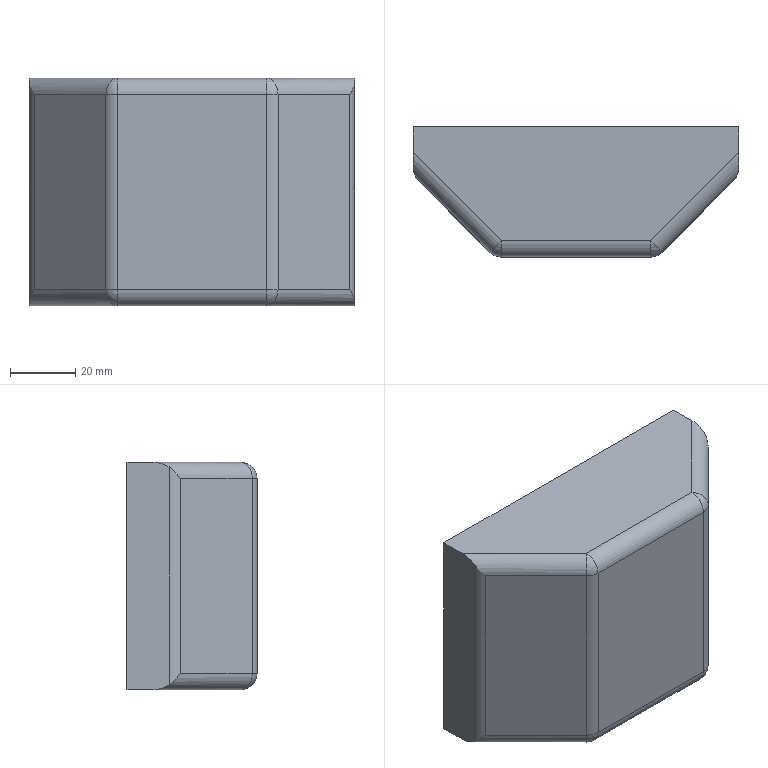Part | SolidWorks | features Extrusion 1, Fillet 1 | 1 solid | 22 faces | box 100 x 40 x 70 mm | volume 234811 mm3 | cylinder 10 | plane 8 | sphere 4 | commonest cylinder face diameters 10 x10
STEP:
#1=CARTESIAN_POINT('',(0.,-12.929,1.464));
#2=VERTEX_POINT('',#1);
#3=CARTESIAN_POINT('',(0.,-12.929,68.536));
#4=VERTEX_POINT('',#3);
#5=CARTESIAN_POINT('',(0.,-12.929,70.));
#6=DIRECTION('',(0.,0.,1.));
#7=VECTOR('',#6,1000.);
#8=LINE('',#5,#7);
#9=EDGE_CURVE('',#2,#4,#8,.T.);
#10=ORIENTED_EDGE('',*,*,#9,.T.);
#11=CARTESIAN_POINT('',(0.,-7.929,70.));
#12=VERTEX_POINT('',#11);
#13=CARTESIAN_POINT('',(0.,-12.929,68.536));
#14=CARTESIAN_POINT('',(0.,-11.585,69.486));
#15=CARTESIAN_POINT('',(0.,-9.829,70.));
#16=CARTESIAN_POINT('',(0.,-7.929,70.));
#17=(BOUNDED_CURVE()B_SPLINE_CURVE(3,(#13,#14,#15,#16),.UNSPECIFIED.,.F.,.F.)B_SPLINE_CURVE_WITH_KNOTS((4,4),(0.7854,1.571),.UNSPECIFIED.)CURVE()GEOMETRIC_REPRESENTATION_ITEM()RATIONAL_B_SPLINE_CURVE((1.,0.9493,0.9493,1.))REPRESENTATION_ITEM(''));
#18=EDGE_CURVE('',#4,#12,#17,.T.);
#19=ORIENTED_EDGE('',*,*,#18,.T.);
#20=CARTESIAN_POINT('',(0.,0.,70.));
#21=VERTEX_POINT('',#20);
#22=CARTESIAN_POINT('',(0.,0.,70.));
#23=DIRECTION('',(0.,-1.,0.));
#24=VECTOR('',#23,1000.);
#25=LINE('',#22,#24);
#26=EDGE_CURVE('',#21,#12,#25,.T.);
#27=ORIENTED_EDGE('',*,*,#26,.F.);
#28=CARTESIAN_POINT('',(0.,0.,0.));
#29=VERTEX_POINT('',#28);
#30=CARTESIAN_POINT('',(0.,0.,70.));
#31=DIRECTION('',(0.,0.,-1.));
#32=VECTOR('',#31,1000.);
#33=LINE('',#30,#32);
#34=EDGE_CURVE('',#21,#29,#33,.T.);
#35=ORIENTED_EDGE('',*,*,#34,.T.);
#36=CARTESIAN_POINT('',(0.,-7.929,0.));
#37=VERTEX_POINT('',#36);
#38=CARTESIAN_POINT('',(0.,0.,0.));
#39=DIRECTION('',(0.,-1.,0.));
#40=VECTOR('',#39,1000.);
#41=LINE('',#38,#40);
#42=EDGE_CURVE('',#29,#37,#41,.T.);
#43=ORIENTED_EDGE('',*,*,#42,.T.);
#44=CARTESIAN_POINT('',(0.,-7.929,0.));
#45=CARTESIAN_POINT('',(0.,-9.829,0.));
#46=CARTESIAN_POINT('',(0.,-11.585,0.5143));
#47=CARTESIAN_POINT('',(0.,-12.929,1.464));
#48=(BOUNDED_CURVE()B_SPLINE_CURVE(3,(#44,#45,#46,#47),.UNSPECIFIED.,.F.,.F.)B_SPLINE_CURVE_WITH_KNOTS((4,4),(1.571,2.356),.UNSPECIFIED.)CURVE()GEOMETRIC_REPRESENTATION_ITEM()RATIONAL_B_SPLINE_CURVE((1.,0.9493,0.9493,1.))REPRESENTATION_ITEM(''));
#49=EDGE_CURVE('',#37,#2,#48,.T.);
#50=ORIENTED_EDGE('',*,*,#49,.T.);
#51=EDGE_LOOP('',(#10,#19,#27,#35,#43,#50));
#52=FACE_OUTER_BOUND('',#51,.T.);
#53=CARTESIAN_POINT('',(0.,0.,70.));
#54=DIRECTION('',(1.,0.,0.));
#55=DIRECTION('',(0.,1.,0.));
#56=AXIS2_PLACEMENT_3D('',#53,#54,#55);
#57=PLANE('',#56);
#58=ADVANCED_FACE('',(#52),#57,.F.);
#59=CARTESIAN_POINT('',(23.536,-38.536,65.));
#60=VERTEX_POINT('',#59);
#61=CARTESIAN_POINT('',(1.464,-16.464,65.));
#62=VERTEX_POINT('',#61);
#63=CARTESIAN_POINT('',(25.,-40.,65.));
#64=DIRECTION('',(-0.7071,0.7071,0.));
#65=VECTOR('',#64,1000.);
#66=LINE('',#63,#65);
#67=EDGE_CURVE('',#60,#62,#66,.T.);
#68=ORIENTED_EDGE('',*,*,#67,.T.);
#69=CARTESIAN_POINT('',(1.464,-16.464,5.));
#70=VERTEX_POINT('',#69);
#71=CARTESIAN_POINT('',(1.464,-16.464,70.));
#72=DIRECTION('',(0.,0.,-1.));
#73=VECTOR('',#72,1000.);
#74=LINE('',#71,#73);
#75=EDGE_CURVE('',#62,#70,#74,.T.);
#76=ORIENTED_EDGE('',*,*,#75,.T.);
#77=CARTESIAN_POINT('',(23.536,-38.536,5.));
#78=VERTEX_POINT('',#77);
#79=CARTESIAN_POINT('',(25.,-40.,5.));
#80=DIRECTION('',(0.7071,-0.7071,0.));
#81=VECTOR('',#80,1000.);
#82=LINE('',#79,#81);
#83=EDGE_CURVE('',#70,#78,#82,.T.);
#84=ORIENTED_EDGE('',*,*,#83,.T.);
#85=CARTESIAN_POINT('',(23.536,-38.536,70.));
#86=DIRECTION('',(0.,0.,1.));
#87=VECTOR('',#86,1000.);
#88=LINE('',#85,#87);
#89=EDGE_CURVE('',#78,#60,#88,.T.);
#90=ORIENTED_EDGE('',*,*,#89,.T.);
#91=EDGE_LOOP('',(#68,#76,#84,#90));
#92=FACE_OUTER_BOUND('',#91,.T.);
#93=CARTESIAN_POINT('',(25.,-40.,70.));
#94=DIRECTION('',(0.7071,0.7071,0.));
#95=DIRECTION('',(-0.7071,0.7071,0.));
#96=AXIS2_PLACEMENT_3D('',#93,#94,#95);
#97=PLANE('',#96);
#98=ADVANCED_FACE('',(#92),#97,.F.);
#99=CARTESIAN_POINT('',(27.071,-40.,65.));
#100=VERTEX_POINT('',#99);
#101=CARTESIAN_POINT('',(27.071,-40.,5.));
#102=VERTEX_POINT('',#101);
#103=CARTESIAN_POINT('',(27.071,-40.,70.));
#104=DIRECTION('',(0.,0.,-1.));
#105=VECTOR('',#104,1000.);
#106=LINE('',#103,#105);
#107=EDGE_CURVE('',#100,#102,#106,.T.);
#108=ORIENTED_EDGE('',*,*,#107,.T.);
#109=CARTESIAN_POINT('',(72.929,-40.,5.));
#110=VERTEX_POINT('',#109);
#111=CARTESIAN_POINT('',(75.,-40.,5.));
#112=DIRECTION('',(1.,0.,0.));
#113=VECTOR('',#112,1000.);
#114=LINE('',#111,#113);
#115=EDGE_CURVE('',#102,#110,#114,.T.);
#116=ORIENTED_EDGE('',*,*,#115,.T.);
#117=CARTESIAN_POINT('',(72.929,-40.,65.));
#118=VERTEX_POINT('',#117);
#119=CARTESIAN_POINT('',(72.929,-40.,70.));
#120=DIRECTION('',(0.,0.,1.));
#121=VECTOR('',#120,1000.);
#122=LINE('',#119,#121);
#123=EDGE_CURVE('',#110,#118,#122,.T.);
#124=ORIENTED_EDGE('',*,*,#123,.T.);
#125=CARTESIAN_POINT('',(50.,-40.,65.));
#126=DIRECTION('',(-1.,0.,0.));
#127=VECTOR('',#126,1000.);
#128=LINE('',#125,#127);
#129=EDGE_CURVE('',#118,#100,#128,.T.);
#130=ORIENTED_EDGE('',*,*,#129,.T.);
#131=EDGE_LOOP('',(#108,#116,#124,#130));
#132=FACE_OUTER_BOUND('',#131,.T.);
#133=CARTESIAN_POINT('',(50.,-40.,70.));
#134=DIRECTION('',(0.,1.,0.));
#135=DIRECTION('',(0.,0.,1.));
#136=AXIS2_PLACEMENT_3D('',#133,#134,#135);
#137=PLANE('',#136);
#138=ADVANCED_FACE('',(#132),#137,.F.);
#139=CARTESIAN_POINT('',(98.536,-16.464,65.));
#140=VERTEX_POINT('',#139);
#141=CARTESIAN_POINT('',(76.464,-38.536,65.));
#142=VERTEX_POINT('',#141);
#143=CARTESIAN_POINT('',(75.,-40.,65.));
#144=DIRECTION('',(-0.7071,-0.7071,0.));
#145=VECTOR('',#144,1000.);
#146=LINE('',#143,#145);
#147=EDGE_CURVE('',#140,#142,#146,.T.);
#148=ORIENTED_EDGE('',*,*,#147,.T.);
#149=CARTESIAN_POINT('',(76.464,-38.536,5.));
#150=VERTEX_POINT('',#149);
#151=CARTESIAN_POINT('',(76.464,-38.536,70.));
#152=DIRECTION('',(0.,0.,-1.));
#153=VECTOR('',#152,1000.);
#154=LINE('',#151,#153);
#155=EDGE_CURVE('',#142,#150,#154,.T.);
#156=ORIENTED_EDGE('',*,*,#155,.T.);
#157=CARTESIAN_POINT('',(98.536,-16.464,5.));
#158=VERTEX_POINT('',#157);
#159=CARTESIAN_POINT('',(100.,-15.,5.));
#160=DIRECTION('',(0.7071,0.7071,0.));
#161=VECTOR('',#160,1000.);
#162=LINE('',#159,#161);
#163=EDGE_CURVE('',#150,#158,#162,.T.);
#164=ORIENTED_EDGE('',*,*,#163,.T.);
#165=CARTESIAN_POINT('',(98.536,-16.464,70.));
#166=DIRECTION('',(0.,0.,1.));
#167=VECTOR('',#166,1000.);
#168=LINE('',#165,#167);
#169=EDGE_CURVE('',#158,#140,#168,.T.);
#170=ORIENTED_EDGE('',*,*,#169,.T.);
#171=EDGE_LOOP('',(#148,#156,#164,#170));
#172=FACE_OUTER_BOUND('',#171,.T.);
#173=CARTESIAN_POINT('',(75.,-40.,70.));
#174=DIRECTION('',(-0.7071,0.7071,0.));
#175=DIRECTION('',(-0.7071,-0.7071,0.));
#176=AXIS2_PLACEMENT_3D('',#173,#174,#175);
#177=PLANE('',#176);
#178=ADVANCED_FACE('',(#172),#177,.F.);
#179=CARTESIAN_POINT('',(100.,-7.929,70.));
#180=VERTEX_POINT('',#179);
#181=CARTESIAN_POINT('',(100.,0.,70.));
#182=VERTEX_POINT('',#181);
#183=CARTESIAN_POINT('',(100.,0.,70.));
#184=DIRECTION('',(0.,1.,0.));
#185=VECTOR('',#184,1000.);
#186=LINE('',#183,#185);
#187=EDGE_CURVE('',#180,#182,#186,.T.);
#188=ORIENTED_EDGE('',*,*,#187,.F.);
#189=CARTESIAN_POINT('',(100.,-12.929,68.536));
#190=VERTEX_POINT('',#189);
#191=CARTESIAN_POINT('',(100.,-7.929,70.));
#192=CARTESIAN_POINT('',(100.,-9.829,70.));
#193=CARTESIAN_POINT('',(100.,-11.585,69.486));
#194=CARTESIAN_POINT('',(100.,-12.929,68.536));
#195=(BOUNDED_CURVE()B_SPLINE_CURVE(3,(#191,#192,#193,#194),.UNSPECIFIED.,.F.,.F.)B_SPLINE_CURVE_WITH_KNOTS((4,4),(1.571,2.356),.UNSPECIFIED.)CURVE()GEOMETRIC_REPRESENTATION_ITEM()RATIONAL_B_SPLINE_CURVE((1.,0.9493,0.9493,1.))REPRESENTATION_ITEM(''));
#196=EDGE_CURVE('',#180,#190,#195,.T.);
#197=ORIENTED_EDGE('',*,*,#196,.T.);
#198=CARTESIAN_POINT('',(100.,-12.929,1.464));
#199=VERTEX_POINT('',#198);
#200=CARTESIAN_POINT('',(100.,-12.929,70.));
#201=DIRECTION('',(0.,0.,-1.));
#202=VECTOR('',#201,1000.);
#203=LINE('',#200,#202);
#204=EDGE_CURVE('',#190,#199,#203,.T.);
#205=ORIENTED_EDGE('',*,*,#204,.T.);
#206=CARTESIAN_POINT('',(100.,-7.929,0.));
#207=VERTEX_POINT('',#206);
#208=CARTESIAN_POINT('',(100.,-12.929,1.464));
#209=CARTESIAN_POINT('',(100.,-11.585,0.5143));
#210=CARTESIAN_POINT('',(100.,-9.829,0.));
#211=CARTESIAN_POINT('',(100.,-7.929,0.));
#212=(BOUNDED_CURVE()B_SPLINE_CURVE(3,(#208,#209,#210,#211),.UNSPECIFIED.,.F.,.F.)B_SPLINE_CURVE_WITH_KNOTS((4,4),(0.7854,1.571),.UNSPECIFIED.)CURVE()GEOMETRIC_REPRESENTATION_ITEM()RATIONAL_B_SPLINE_CURVE((1.,0.9493,0.9493,1.))REPRESENTATION_ITEM(''));
#213=EDGE_CURVE('',#199,#207,#212,.T.);
#214=ORIENTED_EDGE('',*,*,#213,.T.);
#215=CARTESIAN_POINT('',(100.,0.,0.));
#216=VERTEX_POINT('',#215);
#217=CARTESIAN_POINT('',(100.,0.,0.));
#218=DIRECTION('',(0.,1.,0.));
#219=VECTOR('',#218,1000.);
#220=LINE('',#217,#219);
#221=EDGE_CURVE('',#207,#216,#220,.T.);
#222=ORIENTED_EDGE('',*,*,#221,.T.);
#223=CARTESIAN_POINT('',(100.,0.,70.));
#224=DIRECTION('',(0.,0.,-1.));
#225=VECTOR('',#224,1000.);
#226=LINE('',#223,#225);
#227=EDGE_CURVE('',#182,#216,#226,.T.);
#228=ORIENTED_EDGE('',*,*,#227,.F.);
#229=EDGE_LOOP('',(#188,#197,#205,#214,#222,#228));
#230=FACE_OUTER_BOUND('',#229,.T.);
#231=CARTESIAN_POINT('',(100.,0.,70.));
#232=DIRECTION('',(-1.,0.,0.));
#233=DIRECTION('',(0.,0.,1.));
#234=AXIS2_PLACEMENT_3D('',#231,#232,#233);
#235=PLANE('',#234);
#236=ADVANCED_FACE('',(#230),#235,.F.);
#237=CARTESIAN_POINT('',(0.,0.,0.));
#238=DIRECTION('',(-1.,0.,0.));
#239=VECTOR('',#238,1000.);
#240=LINE('',#237,#239);
#241=EDGE_CURVE('',#216,#29,#240,.T.);
#242=ORIENTED_EDGE('',*,*,#241,.T.);
#243=ORIENTED_EDGE('',*,*,#34,.F.);
#244=CARTESIAN_POINT('',(0.,0.,70.));
#245=DIRECTION('',(-1.,0.,0.));
#246=VECTOR('',#245,1000.);
#247=LINE('',#244,#246);
#248=EDGE_CURVE('',#182,#21,#247,.T.);
#249=ORIENTED_EDGE('',*,*,#248,.F.);
#250=ORIENTED_EDGE('',*,*,#227,.T.);
#251=EDGE_LOOP('',(#242,#243,#249,#250));
#252=FACE_OUTER_BOUND('',#251,.T.);
#253=CARTESIAN_POINT('',(0.,0.,70.));
#254=DIRECTION('',(0.,-1.,0.));
#255=DIRECTION('',(0.,0.,-1.));
#256=AXIS2_PLACEMENT_3D('',#253,#254,#255);
#257=PLANE('',#256);
#258=ADVANCED_FACE('',(#252),#257,.F.);
#259=CARTESIAN_POINT('',(27.071,-35.,70.));
#260=VERTEX_POINT('',#259);
#261=CARTESIAN_POINT('',(72.929,-35.,70.));
#262=VERTEX_POINT('',#261);
#263=CARTESIAN_POINT('',(0.,-35.,70.));
#264=DIRECTION('',(1.,0.,0.));
#265=VECTOR('',#264,1000.);
#266=LINE('',#263,#265);
#267=EDGE_CURVE('',#260,#262,#266,.T.);
#268=ORIENTED_EDGE('',*,*,#267,.T.);
#269=CARTESIAN_POINT('',(53.964,-53.964,70.));
#270=DIRECTION('',(0.7071,0.7071,0.));
#271=VECTOR('',#270,1000.);
#272=LINE('',#269,#271);
#273=EDGE_CURVE('',#262,#180,#272,.T.);
#274=ORIENTED_EDGE('',*,*,#273,.T.);
#275=ORIENTED_EDGE('',*,*,#187,.T.);
#276=ORIENTED_EDGE('',*,*,#248,.T.);
#277=ORIENTED_EDGE('',*,*,#26,.T.);
#278=CARTESIAN_POINT('',(-3.964,-3.964,70.));
#279=DIRECTION('',(0.7071,-0.7071,0.));
#280=VECTOR('',#279,1000.);
#281=LINE('',#278,#280);
#282=EDGE_CURVE('',#12,#260,#281,.T.);
#283=ORIENTED_EDGE('',*,*,#282,.T.);
#284=EDGE_LOOP('',(#268,#274,#275,#276,#277,#283));
#285=FACE_OUTER_BOUND('',#284,.T.);
#286=CARTESIAN_POINT('',(0.,0.,70.));
#287=DIRECTION('',(0.,0.,-1.));
#288=DIRECTION('',(-1.,0.,0.));
#289=AXIS2_PLACEMENT_3D('',#286,#287,#288);
#290=PLANE('',#289);
#291=ADVANCED_FACE('',(#285),#290,.F.);
#292=ORIENTED_EDGE('',*,*,#221,.F.);
#293=CARTESIAN_POINT('',(72.929,-35.,0.));
#294=VERTEX_POINT('',#293);
#295=CARTESIAN_POINT('',(71.464,-36.464,0.));
#296=DIRECTION('',(-0.7071,-0.7071,0.));
#297=VECTOR('',#296,1000.);
#298=LINE('',#295,#297);
#299=EDGE_CURVE('',#207,#294,#298,.T.);
#300=ORIENTED_EDGE('',*,*,#299,.T.);
#301=CARTESIAN_POINT('',(27.071,-35.,0.));
#302=VERTEX_POINT('',#301);
#303=CARTESIAN_POINT('',(25.,-35.,0.));
#304=DIRECTION('',(-1.,0.,0.));
#305=VECTOR('',#304,1000.);
#306=LINE('',#303,#305);
#307=EDGE_CURVE('',#294,#302,#306,.T.);
#308=ORIENTED_EDGE('',*,*,#307,.T.);
#309=CARTESIAN_POINT('',(3.536,-11.464,0.));
#310=DIRECTION('',(-0.7071,0.7071,0.));
#311=VECTOR('',#310,1000.);
#312=LINE('',#309,#311);
#313=EDGE_CURVE('',#302,#37,#312,.T.);
#314=ORIENTED_EDGE('',*,*,#313,.T.);
#315=ORIENTED_EDGE('',*,*,#42,.F.);
#316=ORIENTED_EDGE('',*,*,#241,.F.);
#317=EDGE_LOOP('',(#292,#300,#308,#314,#315,#316));
#318=FACE_OUTER_BOUND('',#317,.T.);
#319=CARTESIAN_POINT('',(0.,0.,0.));
#320=DIRECTION('',(0.,0.,-1.));
#321=DIRECTION('',(-1.,0.,0.));
#322=AXIS2_PLACEMENT_3D('',#319,#320,#321);
#323=PLANE('',#322);
#324=ADVANCED_FACE('',(#318),#323,.T.);
#325=CARTESIAN_POINT('',(1.464,-16.464,5.));
#326=CARTESIAN_POINT('',(0.5143,-15.514,3.656));
#327=CARTESIAN_POINT('',(0.,-14.273,2.415));
#328=CARTESIAN_POINT('',(0.,-12.929,1.464));
#329=(BOUNDED_CURVE()B_SPLINE_CURVE(3,(#325,#326,#327,#328),.UNSPECIFIED.,.F.,.F.)B_SPLINE_CURVE_WITH_KNOTS((4,4),(4.712,5.498),.UNSPECIFIED.)CURVE()GEOMETRIC_REPRESENTATION_ITEM()RATIONAL_B_SPLINE_CURVE((1.,0.9493,0.9493,1.))REPRESENTATION_ITEM(''));
#330=EDGE_CURVE('',#70,#2,#329,.T.);
#331=ORIENTED_EDGE('',*,*,#330,.F.);
#332=ORIENTED_EDGE('',*,*,#75,.F.);
#333=CARTESIAN_POINT('',(0.,-12.929,68.536));
#334=CARTESIAN_POINT('',(0.,-14.273,67.585));
#335=CARTESIAN_POINT('',(0.5143,-15.514,66.344));
#336=CARTESIAN_POINT('',(1.464,-16.464,65.));
#337=(BOUNDED_CURVE()B_SPLINE_CURVE(3,(#333,#334,#335,#336),.UNSPECIFIED.,.F.,.F.)B_SPLINE_CURVE_WITH_KNOTS((4,4),(3.927,4.712),.UNSPECIFIED.)CURVE()GEOMETRIC_REPRESENTATION_ITEM()RATIONAL_B_SPLINE_CURVE((1.,0.9493,0.9493,1.))REPRESENTATION_ITEM(''));
#338=EDGE_CURVE('',#4,#62,#337,.T.);
#339=ORIENTED_EDGE('',*,*,#338,.F.);
#340=ORIENTED_EDGE('',*,*,#9,.F.);
#341=EDGE_LOOP('',(#331,#332,#339,#340));
#342=FACE_OUTER_BOUND('',#341,.T.);
#343=CARTESIAN_POINT('',(5.,-12.929,70.));
#344=DIRECTION('',(0.,0.,-1.));
#345=DIRECTION('',(-1.,0.,0.));
#346=AXIS2_PLACEMENT_3D('',#343,#344,#345);
#347=CYLINDRICAL_SURFACE('',#346,5.);
#348=ADVANCED_FACE('',(#342),#347,.T.);
#349=ORIENTED_EDGE('',*,*,#338,.T.);
#350=ORIENTED_EDGE('',*,*,#67,.F.);
#351=CARTESIAN_POINT('',(27.071,-35.,65.));
#352=DIRECTION('',(0.7071,-0.7071,0.));
#353=DIRECTION('',(0.7071,0.7071,0.));
#354=AXIS2_PLACEMENT_3D('',#351,#352,#353);
#355=CIRCLE('',#354,5.);
#356=EDGE_CURVE('',#260,#60,#355,.T.);
#357=ORIENTED_EDGE('',*,*,#356,.F.);
#358=ORIENTED_EDGE('',*,*,#282,.F.);
#359=ORIENTED_EDGE('',*,*,#18,.F.);
#360=EDGE_LOOP('',(#349,#350,#357,#358,#359));
#361=FACE_OUTER_BOUND('',#360,.T.);
#362=CARTESIAN_POINT('',(-3.964,-3.964,65.));
#363=DIRECTION('',(0.7071,-0.7071,0.));
#364=DIRECTION('',(0.7071,0.7071,0.));
#365=AXIS2_PLACEMENT_3D('',#362,#363,#364);
#366=CYLINDRICAL_SURFACE('',#365,5.);
#367=ADVANCED_FACE('',(#361),#366,.T.);
#368=ORIENTED_EDGE('',*,*,#49,.F.);
#369=ORIENTED_EDGE('',*,*,#313,.F.);
#370=CARTESIAN_POINT('',(27.071,-35.,5.));
#371=DIRECTION('',(0.7071,-0.7071,0.));
#372=DIRECTION('',(0.7071,0.7071,0.));
#373=AXIS2_PLACEMENT_3D('',#370,#371,#372);
#374=CIRCLE('',#373,5.);
#375=EDGE_CURVE('',#78,#302,#374,.T.);
#376=ORIENTED_EDGE('',*,*,#375,.F.);
#377=ORIENTED_EDGE('',*,*,#83,.F.);
#378=ORIENTED_EDGE('',*,*,#330,.T.);
#379=EDGE_LOOP('',(#368,#369,#376,#377,#378));
#380=FACE_OUTER_BOUND('',#379,.T.);
#381=CARTESIAN_POINT('',(28.536,-36.464,5.));
#382=DIRECTION('',(-0.7071,0.7071,0.));
#383=DIRECTION('',(-0.7071,-0.7071,0.));
#384=AXIS2_PLACEMENT_3D('',#381,#382,#383);
#385=CYLINDRICAL_SURFACE('',#384,5.);
#386=ADVANCED_FACE('',(#380),#385,.T.);
#387=CARTESIAN_POINT('',(27.071,-35.,65.));
#388=DIRECTION('',(0.,0.,1.));
#389=DIRECTION('',(1.,0.,0.));
#390=AXIS2_PLACEMENT_3D('',#387,#388,#389);
#391=CIRCLE('',#390,5.);
#392=EDGE_CURVE('',#60,#100,#391,.T.);
#393=ORIENTED_EDGE('',*,*,#392,.F.);
#394=ORIENTED_EDGE('',*,*,#89,.F.);
#395=CARTESIAN_POINT('',(27.071,-35.,5.));
#396=DIRECTION('',(0.,0.,-1.));
#397=DIRECTION('',(-1.,0.,0.));
#398=AXIS2_PLACEMENT_3D('',#395,#396,#397);
#399=CIRCLE('',#398,5.);
#400=EDGE_CURVE('',#102,#78,#399,.T.);
#401=ORIENTED_EDGE('',*,*,#400,.F.);
#402=ORIENTED_EDGE('',*,*,#107,.F.);
#403=EDGE_LOOP('',(#393,#394,#401,#402));
#404=FACE_OUTER_BOUND('',#403,.T.);
#405=CARTESIAN_POINT('',(27.071,-35.,70.));
#406=DIRECTION('',(0.,0.,-1.));
#407=DIRECTION('',(-1.,0.,0.));
#408=AXIS2_PLACEMENT_3D('',#405,#406,#407);
#409=CYLINDRICAL_SURFACE('',#408,5.);
#410=ADVANCED_FACE('',(#404),#409,.T.);
#411=ORIENTED_EDGE('',*,*,#356,.T.);
#412=ORIENTED_EDGE('',*,*,#392,.T.);
#413=CARTESIAN_POINT('',(27.071,-35.,65.));
#414=DIRECTION('',(1.,0.,0.));
#415=DIRECTION('',(0.,0.,1.));
#416=AXIS2_PLACEMENT_3D('',#413,#414,#415);
#417=CIRCLE('',#416,5.);
#418=EDGE_CURVE('',#260,#100,#417,.T.);
#419=ORIENTED_EDGE('',*,*,#418,.F.);
#420=EDGE_LOOP('',(#411,#412,#419));
#421=FACE_OUTER_BOUND('',#420,.T.);
#422=CARTESIAN_POINT('',(27.071,-35.,65.));
#423=DIRECTION('',(0.,1.,0.));
#424=DIRECTION('',(1.,0.,0.));
#425=AXIS2_PLACEMENT_3D('',#422,#423,#424);
#426=SPHERICAL_SURFACE('',#425,5.);
#427=ADVANCED_FACE('',(#421),#426,.T.);
#428=CARTESIAN_POINT('',(100.,-12.929,1.464));
#429=CARTESIAN_POINT('',(100.,-14.273,2.415));
#430=CARTESIAN_POINT('',(99.486,-15.514,3.656));
#431=CARTESIAN_POINT('',(98.536,-16.464,5.));
#432=(BOUNDED_CURVE()B_SPLINE_CURVE(3,(#428,#429,#430,#431),.UNSPECIFIED.,.F.,.F.)B_SPLINE_CURVE_WITH_KNOTS((4,4),(3.927,4.712),.UNSPECIFIED.)CURVE()GEOMETRIC_REPRESENTATION_ITEM()RATIONAL_B_SPLINE_CURVE((1.,0.9493,0.9493,1.))REPRESENTATION_ITEM(''));
#433=EDGE_CURVE('',#199,#158,#432,.T.);
#434=ORIENTED_EDGE('',*,*,#433,.F.);
#435=ORIENTED_EDGE('',*,*,#204,.F.);
#436=CARTESIAN_POINT('',(98.536,-16.464,65.));
#437=CARTESIAN_POINT('',(99.486,-15.514,66.344));
#438=CARTESIAN_POINT('',(100.,-14.273,67.585));
#439=CARTESIAN_POINT('',(100.,-12.929,68.536));
#440=(BOUNDED_CURVE()B_SPLINE_CURVE(3,(#436,#437,#438,#439),.UNSPECIFIED.,.F.,.F.)B_SPLINE_CURVE_WITH_KNOTS((4,4),(1.571,2.356),.UNSPECIFIED.)CURVE()GEOMETRIC_REPRESENTATION_ITEM()RATIONAL_B_SPLINE_CURVE((1.,0.9493,0.9493,1.))REPRESENTATION_ITEM(''));
#441=EDGE_CURVE('',#140,#190,#440,.T.);
#442=ORIENTED_EDGE('',*,*,#441,.F.);
#443=ORIENTED_EDGE('',*,*,#169,.F.);
#444=EDGE_LOOP('',(#434,#435,#442,#443));
#445=FACE_OUTER_BOUND('',#444,.T.);
#446=CARTESIAN_POINT('',(95.,-12.929,70.));
#447=DIRECTION('',(0.,0.,-1.));
#448=DIRECTION('',(-1.,0.,0.));
#449=AXIS2_PLACEMENT_3D('',#446,#447,#448);
#450=CYLINDRICAL_SURFACE('',#449,5.);
#451=ADVANCED_FACE('',(#445),#450,.T.);
#452=ORIENTED_EDGE('',*,*,#400,.T.);
#453=ORIENTED_EDGE('',*,*,#375,.T.);
#454=CARTESIAN_POINT('',(27.071,-35.,5.));
#455=DIRECTION('',(1.,0.,0.));
#456=DIRECTION('',(0.,-1.,0.));
#457=AXIS2_PLACEMENT_3D('',#454,#455,#456);
#458=CIRCLE('',#457,5.);
#459=EDGE_CURVE('',#102,#302,#458,.T.);
#460=ORIENTED_EDGE('',*,*,#459,.F.);
#461=EDGE_LOOP('',(#452,#453,#460));
#462=FACE_OUTER_BOUND('',#461,.T.);
#463=CARTESIAN_POINT('',(27.071,-35.,5.));
#464=DIRECTION('',(0.,1.,0.));
#465=DIRECTION('',(1.,0.,0.));
#466=AXIS2_PLACEMENT_3D('',#463,#464,#465);
#467=SPHERICAL_SURFACE('',#466,5.);
#468=ADVANCED_FACE('',(#462),#467,.T.);
#469=ORIENTED_EDGE('',*,*,#418,.T.);
#470=ORIENTED_EDGE('',*,*,#129,.F.);
#471=CARTESIAN_POINT('',(72.929,-35.,65.));
#472=DIRECTION('',(1.,0.,0.));
#473=DIRECTION('',(0.,1.,0.));
#474=AXIS2_PLACEMENT_3D('',#471,#472,#473);
#475=CIRCLE('',#474,5.);
#476=EDGE_CURVE('',#262,#118,#475,.T.);
#477=ORIENTED_EDGE('',*,*,#476,.F.);
#478=ORIENTED_EDGE('',*,*,#267,.F.);
#479=EDGE_LOOP('',(#469,#470,#477,#478));
#480=FACE_OUTER_BOUND('',#479,.T.);
#481=CARTESIAN_POINT('',(0.,-35.,65.));
#482=DIRECTION('',(1.,0.,0.));
#483=DIRECTION('',(0.,0.,-1.));
#484=AXIS2_PLACEMENT_3D('',#481,#482,#483);
#485=CYLINDRICAL_SURFACE('',#484,5.);
#486=ADVANCED_FACE('',(#480),#485,.T.);
#487=ORIENTED_EDGE('',*,*,#196,.F.);
#488=ORIENTED_EDGE('',*,*,#273,.F.);
#489=CARTESIAN_POINT('',(72.929,-35.,65.));
#490=DIRECTION('',(-0.7071,-0.7071,0.));
#491=DIRECTION('',(0.7071,-0.7071,0.));
#492=AXIS2_PLACEMENT_3D('',#489,#490,#491);
#493=CIRCLE('',#492,5.);
#494=EDGE_CURVE('',#142,#262,#493,.T.);
#495=ORIENTED_EDGE('',*,*,#494,.F.);
#496=ORIENTED_EDGE('',*,*,#147,.F.);
#497=ORIENTED_EDGE('',*,*,#441,.T.);
#498=EDGE_LOOP('',(#487,#488,#495,#496,#497));
#499=FACE_OUTER_BOUND('',#498,.T.);
#500=CARTESIAN_POINT('',(53.964,-53.964,65.));
#501=DIRECTION('',(0.7071,0.7071,0.));
#502=DIRECTION('',(-0.7071,0.7071,0.));
#503=AXIS2_PLACEMENT_3D('',#500,#501,#502);
#504=CYLINDRICAL_SURFACE('',#503,5.);
#505=ADVANCED_FACE('',(#499),#504,.T.);
#506=ORIENTED_EDGE('',*,*,#433,.T.);
#507=ORIENTED_EDGE('',*,*,#163,.F.);
#508=CARTESIAN_POINT('',(72.929,-35.,5.));
#509=DIRECTION('',(-0.7071,-0.7071,0.));
#510=DIRECTION('',(0.7071,-0.7071,0.));
#511=AXIS2_PLACEMENT_3D('',#508,#509,#510);
#512=CIRCLE('',#511,5.);
#513=EDGE_CURVE('',#294,#150,#512,.T.);
#514=ORIENTED_EDGE('',*,*,#513,.F.);
#515=ORIENTED_EDGE('',*,*,#299,.F.);
#516=ORIENTED_EDGE('',*,*,#213,.F.);
#517=EDGE_LOOP('',(#506,#507,#514,#515,#516));
#518=FACE_OUTER_BOUND('',#517,.T.);
#519=CARTESIAN_POINT('',(71.464,-36.464,5.));
#520=DIRECTION('',(-0.7071,-0.7071,0.));
#521=DIRECTION('',(0.7071,-0.7071,0.));
#522=AXIS2_PLACEMENT_3D('',#519,#520,#521);
#523=CYLINDRICAL_SURFACE('',#522,5.);
#524=ADVANCED_FACE('',(#518),#523,.T.);
#525=ORIENTED_EDGE('',*,*,#459,.T.);
#526=ORIENTED_EDGE('',*,*,#307,.F.);
#527=CARTESIAN_POINT('',(72.929,-35.,5.));
#528=DIRECTION('',(1.,0.,0.));
#529=DIRECTION('',(0.,0.,-1.));
#530=AXIS2_PLACEMENT_3D('',#527,#528,#529);
#531=CIRCLE('',#530,5.);
#532=EDGE_CURVE('',#110,#294,#531,.T.);
#533=ORIENTED_EDGE('',*,*,#532,.F.);
#534=ORIENTED_EDGE('',*,*,#115,.F.);
#535=EDGE_LOOP('',(#525,#526,#533,#534));
#536=FACE_OUTER_BOUND('',#535,.T.);
#537=CARTESIAN_POINT('',(50.,-35.,5.));
#538=DIRECTION('',(-1.,0.,0.));
#539=DIRECTION('',(0.,0.,1.));
#540=AXIS2_PLACEMENT_3D('',#537,#538,#539);
#541=CYLINDRICAL_SURFACE('',#540,5.);
#542=ADVANCED_FACE('',(#536),#541,.T.);
#543=ORIENTED_EDGE('',*,*,#494,.T.);
#544=ORIENTED_EDGE('',*,*,#476,.T.);
#545=CARTESIAN_POINT('',(72.929,-35.,65.));
#546=DIRECTION('',(0.,0.,-1.));
#547=DIRECTION('',(1.,0.,0.));
#548=AXIS2_PLACEMENT_3D('',#545,#546,#547);
#549=CIRCLE('',#548,5.);
#550=EDGE_CURVE('',#142,#118,#549,.T.);
#551=ORIENTED_EDGE('',*,*,#550,.F.);
#552=EDGE_LOOP('',(#543,#544,#551));
#553=FACE_OUTER_BOUND('',#552,.T.);
#554=CARTESIAN_POINT('',(72.929,-35.,65.));
#555=DIRECTION('',(0.,1.,0.));
#556=DIRECTION('',(1.,0.,0.));
#557=AXIS2_PLACEMENT_3D('',#554,#555,#556);
#558=SPHERICAL_SURFACE('',#557,5.);
#559=ADVANCED_FACE('',(#553),#558,.T.);
#560=ORIENTED_EDGE('',*,*,#532,.T.);
#561=ORIENTED_EDGE('',*,*,#513,.T.);
#562=CARTESIAN_POINT('',(72.929,-35.,5.));
#563=DIRECTION('',(0.,0.,1.));
#564=DIRECTION('',(-1.,0.,0.));
#565=AXIS2_PLACEMENT_3D('',#562,#563,#564);
#566=CIRCLE('',#565,5.);
#567=EDGE_CURVE('',#110,#150,#566,.T.);
#568=ORIENTED_EDGE('',*,*,#567,.F.);
#569=EDGE_LOOP('',(#560,#561,#568));
#570=FACE_OUTER_BOUND('',#569,.T.);
#571=CARTESIAN_POINT('',(72.929,-35.,5.));
#572=DIRECTION('',(0.,1.,0.));
#573=DIRECTION('',(1.,0.,0.));
#574=AXIS2_PLACEMENT_3D('',#571,#572,#573);
#575=SPHERICAL_SURFACE('',#574,5.);
#576=ADVANCED_FACE('',(#570),#575,.T.);
#577=ORIENTED_EDGE('',*,*,#550,.T.);
#578=ORIENTED_EDGE('',*,*,#123,.F.);
#579=ORIENTED_EDGE('',*,*,#567,.T.);
#580=ORIENTED_EDGE('',*,*,#155,.F.);
#581=EDGE_LOOP('',(#577,#578,#579,#580));
#582=FACE_OUTER_BOUND('',#581,.T.);
#583=CARTESIAN_POINT('',(72.929,-35.,70.));
#584=DIRECTION('',(0.,0.,-1.));
#585=DIRECTION('',(-1.,0.,0.));
#586=AXIS2_PLACEMENT_3D('',#583,#584,#585);
#587=CYLINDRICAL_SURFACE('',#586,5.);
#588=ADVANCED_FACE('',(#582),#587,.T.);
#589=CLOSED_SHELL('',(#58,#98,#138,#178,#236,#258,#291,#324,#348,#367,#386,#410,#427,#451,#468,#486,#505,#524,#542,#559,#576,#588));
#590=MANIFOLD_SOLID_BREP('',#589);
#591=CARTESIAN_POINT('',(0.,0.,0.));
#592=DIRECTION('',(0.,0.,1.));
#593=DIRECTION('',(1.,0.,0.));
#594=AXIS2_PLACEMENT_3D('',#591,#592,#593);
#595=(LENGTH_UNIT()NAMED_UNIT(*)SI_UNIT(.MILLI.,.METRE.));
#596=UNCERTAINTY_MEASURE_WITH_UNIT(LENGTH_MEASURE(0.00001),#595,'','');
#597=(NAMED_UNIT(*)PLANE_ANGLE_UNIT()SI_UNIT($,.RADIAN.));
#598=(NAMED_UNIT(*)SI_UNIT($,.STERADIAN.)SOLID_ANGLE_UNIT());
#599=(GEOMETRIC_REPRESENTATION_CONTEXT(3)GLOBAL_UNCERTAINTY_ASSIGNED_CONTEXT((#596))GLOBAL_UNIT_ASSIGNED_CONTEXT((#595,#597,#598))REPRESENTATION_CONTEXT('',''));
#600=ADVANCED_BREP_SHAPE_REPRESENTATION('',(#590,#594),#599);